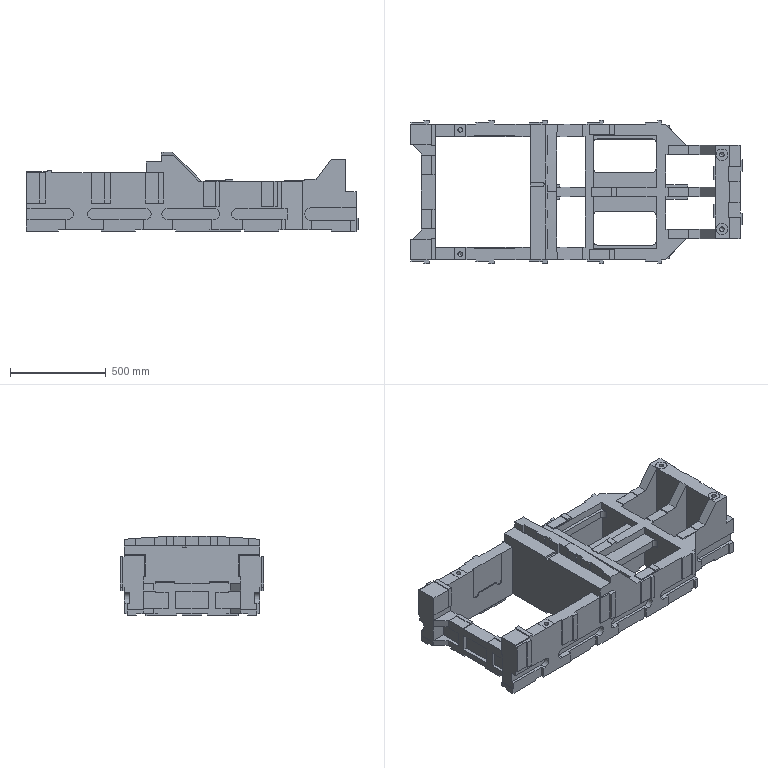Part | NX | features MAIN_BODY 2 | 1 solid | 495 faces | box 1738 x 750 x 415.845 mm | volume 127984690 mm3 | plane 457 | cylinder 33 | cone 3 | spline 2 | commonest cylinder face diameters 40 x12 55 x12 24 x4 60 x2 65 x2 20 x1